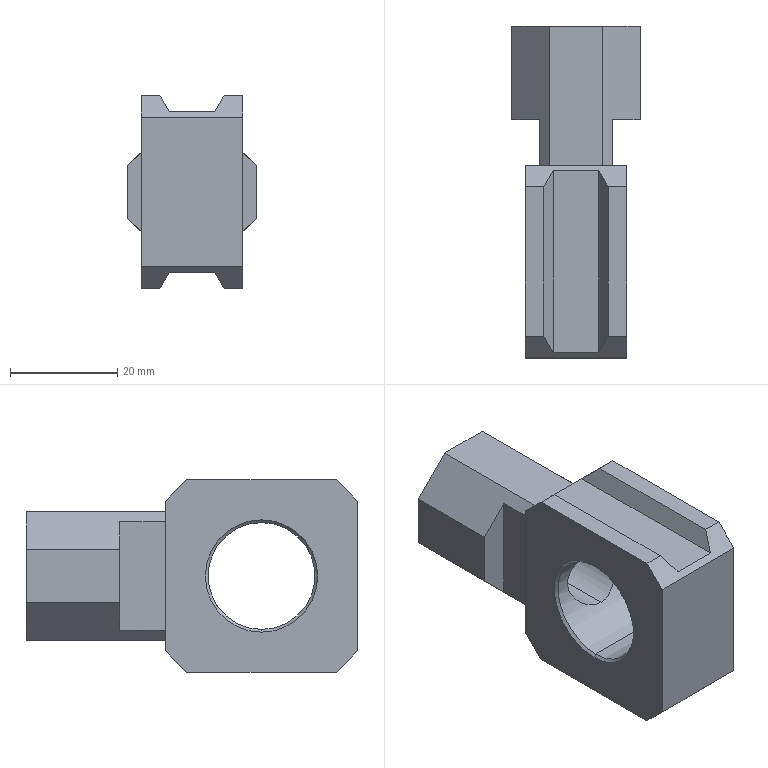Part | STEP file | AC40-04-KSTV-38JNR_AC3009A T Interface-1 | 1 solid | 44 faces | box 24 x 62 x 36 mm | volume 21819 mm3 | plane 32 | cone 8 | cylinder 4 | commonest cylinder face diameters 13 x2 20 x2